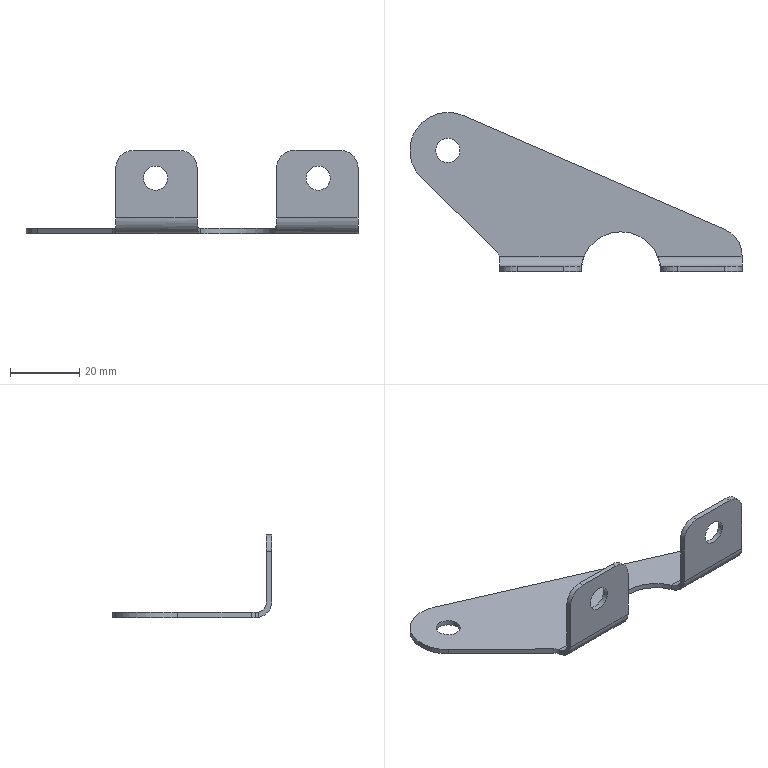Part | NX | features SKETCH 4, DATUM_CSYS 3, DATUM_PLANE 2, EXTRUDE 2, Flange 2, BLEND 1, Base Tab 1 | 1 solid | 35 faces | box 96 x 46 x 24 mm | volume 4607 mm3 | plane 16 | cylinder 15 | spline 4 | commonest cylinder face diameters 10 x4 6 x3 7 x3 9 x2 16 x1 22 x1
STEP:
#1=CARTESIAN_POINT('',(10.583,4.5,0.));
#2=VERTEX_POINT('',#1);
#3=CARTESIAN_POINT('',(-10.583,4.5,0.));
#4=VERTEX_POINT('',#3);
#5=CARTESIAN_POINT('',(0.,0.,0.));
#6=DIRECTION('',(0.,0.,1.));
#7=DIRECTION('',(1.,0.,0.));
#8=AXIS2_PLACEMENT_3D('',#5,#6,#7);
#9=CIRCLE('',#8,11.5);
#10=EDGE_CURVE('',#2,#4,#9,.T.);
#11=ORIENTED_EDGE('',*,*,#10,.F.);
#12=CARTESIAN_POINT('',(10.583,4.5,1.5));
#13=VERTEX_POINT('',#12);
#14=CARTESIAN_POINT('',(10.583,4.5,1.5));
#15=DIRECTION('',(0.,0.,-1.));
#16=VECTOR('',#15,1000.);
#17=LINE('',#14,#16);
#18=EDGE_CURVE('',#13,#2,#17,.T.);
#19=ORIENTED_EDGE('',*,*,#18,.F.);
#20=CARTESIAN_POINT('',(-10.583,4.5,1.5));
#21=VERTEX_POINT('',#20);
#22=CARTESIAN_POINT('',(0.,0.,1.5));
#23=DIRECTION('',(0.,0.,1.));
#24=DIRECTION('',(1.,0.,0.));
#25=AXIS2_PLACEMENT_3D('',#22,#23,#24);
#26=CIRCLE('',#25,11.5);
#27=EDGE_CURVE('',#13,#21,#26,.T.);
#28=ORIENTED_EDGE('',*,*,#27,.T.);
#29=CARTESIAN_POINT('',(-10.583,4.5,1.5));
#30=DIRECTION('',(0.,0.,-1.));
#31=VECTOR('',#30,1000.);
#32=LINE('',#29,#31);
#33=EDGE_CURVE('',#21,#4,#32,.T.);
#34=ORIENTED_EDGE('',*,*,#33,.T.);
#35=EDGE_LOOP('',(#11,#19,#28,#34));
#36=FACE_BOUND('',#35,.T.);
#37=CARTESIAN_POINT('',(0.,0.,1.5));
#38=DIRECTION('',(0.,0.,-1.));
#39=DIRECTION('',(-1.,0.,0.));
#40=AXIS2_PLACEMENT_3D('',#37,#38,#39);
#41=CYLINDRICAL_SURFACE('',#40,11.5);
#42=ADVANCED_FACE('',(#36),#41,.F.);
#43=CARTESIAN_POINT('',(35.,1.5,19.));
#44=VERTEX_POINT('',#43);
#45=CARTESIAN_POINT('',(35.,1.5,4.5));
#46=VERTEX_POINT('',#45);
#47=CARTESIAN_POINT('',(35.,1.5,24.));
#48=DIRECTION('',(0.,0.,-1.));
#49=VECTOR('',#48,1000.);
#50=LINE('',#47,#49);
#51=EDGE_CURVE('',#44,#46,#50,.T.);
#52=ORIENTED_EDGE('',*,*,#51,.F.);
#53=CARTESIAN_POINT('',(35.,0.,19.));
#54=VERTEX_POINT('',#53);
#55=CARTESIAN_POINT('',(35.,4.757,19.));
#56=DIRECTION('',(0.,1.,0.));
#57=VECTOR('',#56,1000.);
#58=LINE('',#55,#57);
#59=EDGE_CURVE('',#44,#54,#58,.F.);
#60=ORIENTED_EDGE('',*,*,#59,.T.);
#61=CARTESIAN_POINT('',(35.,0.,4.5));
#62=VERTEX_POINT('',#61);
#63=CARTESIAN_POINT('',(35.,0.,24.));
#64=DIRECTION('',(0.,0.,-1.));
#65=VECTOR('',#64,1000.);
#66=LINE('',#63,#65);
#67=EDGE_CURVE('',#54,#62,#66,.T.);
#68=ORIENTED_EDGE('',*,*,#67,.T.);
#69=CARTESIAN_POINT('',(35.,4.5,0.));
#70=VERTEX_POINT('',#69);
#71=CARTESIAN_POINT('',(35.,4.5,4.5));
#72=DIRECTION('',(-1.,0.,0.));
#73=DIRECTION('',(0.,0.,1.));
#74=AXIS2_PLACEMENT_3D('',#71,#72,#73);
#75=CIRCLE('',#74,4.5);
#76=EDGE_CURVE('',#70,#62,#75,.T.);
#77=ORIENTED_EDGE('',*,*,#76,.F.);
#78=CARTESIAN_POINT('',(35.,4.757,0.));
#79=VERTEX_POINT('',#78);
#80=CARTESIAN_POINT('',(35.,4.757,0.));
#81=DIRECTION('',(0.,-1.,0.));
#82=VECTOR('',#81,1000.);
#83=LINE('',#80,#82);
#84=EDGE_CURVE('',#79,#70,#83,.T.);
#85=ORIENTED_EDGE('',*,*,#84,.F.);
#86=CARTESIAN_POINT('',(35.,4.757,1.5));
#87=VERTEX_POINT('',#86);
#88=CARTESIAN_POINT('',(35.,4.757,1.5));
#89=DIRECTION('',(0.,0.,-1.));
#90=VECTOR('',#89,1000.);
#91=LINE('',#88,#90);
#92=EDGE_CURVE('',#87,#79,#91,.T.);
#93=ORIENTED_EDGE('',*,*,#92,.F.);
#94=CARTESIAN_POINT('',(35.,4.5,1.5));
#95=VERTEX_POINT('',#94);
#96=CARTESIAN_POINT('',(35.,4.757,1.5));
#97=DIRECTION('',(0.,-1.,0.));
#98=VECTOR('',#97,1000.);
#99=LINE('',#96,#98);
#100=EDGE_CURVE('',#87,#95,#99,.T.);
#101=ORIENTED_EDGE('',*,*,#100,.T.);
#102=CARTESIAN_POINT('',(35.,4.5,4.5));
#103=DIRECTION('',(-1.,0.,0.));
#104=DIRECTION('',(0.,-1.,0.));
#105=AXIS2_PLACEMENT_3D('',#102,#103,#104);
#106=CIRCLE('',#105,3.);
#107=EDGE_CURVE('',#95,#46,#106,.T.);
#108=ORIENTED_EDGE('',*,*,#107,.T.);
#109=EDGE_LOOP('',(#52,#60,#68,#77,#85,#93,#101,#108));
#110=FACE_BOUND('',#109,.T.);
#111=CARTESIAN_POINT('',(35.,4.757,1.5));
#112=DIRECTION('',(1.,0.,0.));
#113=DIRECTION('',(0.,0.,-1.));
#114=AXIS2_PLACEMENT_3D('',#111,#112,#113);
#115=PLANE('',#114);
#116=ADVANCED_FACE('',(#110),#115,.T.);
#117=CARTESIAN_POINT('',(-46.5,35.,0.));
#118=VERTEX_POINT('',#117);
#119=CARTESIAN_POINT('',(-50.,35.,0.));
#120=DIRECTION('',(0.,0.,1.));
#121=DIRECTION('',(1.,0.,0.));
#122=AXIS2_PLACEMENT_3D('',#119,#120,#121);
#123=CIRCLE('',#122,3.5);
#124=EDGE_CURVE('',#118,#118,#123,.T.);
#125=ORIENTED_EDGE('',*,*,#124,.T.);
#126=EDGE_LOOP('',(#125));
#127=FACE_BOUND('',#126,.T.);
#128=ORIENTED_EDGE('',*,*,#84,.T.);
#129=CARTESIAN_POINT('',(35.,4.5,0.));
#130=DIRECTION('',(-1.,0.,0.));
#131=VECTOR('',#130,1000.);
#132=LINE('',#129,#131);
#133=EDGE_CURVE('',#70,#2,#132,.T.);
#134=ORIENTED_EDGE('',*,*,#133,.T.);
#135=ORIENTED_EDGE('',*,*,#10,.T.);
#136=CARTESIAN_POINT('',(-35.,4.5,0.));
#137=VERTEX_POINT('',#136);
#138=CARTESIAN_POINT('',(-35.002,4.5,0.));
#139=DIRECTION('',(-1.,0.,0.));
#140=VECTOR('',#139,1000.);
#141=LINE('',#138,#140);
#142=EDGE_CURVE('',#4,#137,#141,.T.);
#143=ORIENTED_EDGE('',*,*,#142,.T.);
#144=CARTESIAN_POINT('',(-35.002,4.5,0.));
#145=VERTEX_POINT('',#144);
#146=CARTESIAN_POINT('',(-35.002,4.5,0.));
#147=DIRECTION('',(-1.,0.,0.));
#148=VECTOR('',#147,1000.);
#149=LINE('',#146,#148);
#150=EDGE_CURVE('',#137,#145,#149,.T.);
#151=ORIENTED_EDGE('',*,*,#150,.T.);
#152=CARTESIAN_POINT('',(-35.002,3.845,0.));
#153=VERTEX_POINT('',#152);
#154=CARTESIAN_POINT('',(-35.002,0.,0.));
#155=DIRECTION('',(0.,-1.,0.));
#156=VECTOR('',#155,1000.);
#157=LINE('',#154,#156);
#158=EDGE_CURVE('',#145,#153,#157,.T.);
#159=ORIENTED_EDGE('',*,*,#158,.T.);
#160=CARTESIAN_POINT('',(-35.905,5.883,0.));
#161=VERTEX_POINT('',#160);
#162=CARTESIAN_POINT('',(-38.,3.736,0.));
#163=DIRECTION('',(0.,0.,1.));
#164=DIRECTION('',(1.,0.,0.));
#165=AXIS2_PLACEMENT_3D('',#162,#163,#164);
#166=CIRCLE('',#165,3.);
#167=EDGE_CURVE('',#153,#161,#166,.T.);
#168=ORIENTED_EDGE('',*,*,#167,.T.);
#169=CARTESIAN_POINT('',(-57.681,27.126,0.));
#170=VERTEX_POINT('',#169);
#171=CARTESIAN_POINT('',(-35.905,5.883,0.));
#172=DIRECTION('',(-0.7158,0.6983,0.));
#173=VECTOR('',#172,1000.);
#174=LINE('',#171,#173);
#175=EDGE_CURVE('',#161,#170,#174,.T.);
#176=ORIENTED_EDGE('',*,*,#175,.T.);
#177=CARTESIAN_POINT('',(-45.61,45.086,0.));
#178=VERTEX_POINT('',#177);
#179=CARTESIAN_POINT('',(-50.,35.,0.));
#180=DIRECTION('',(0.,0.,-1.));
#181=DIRECTION('',(1.,0.,0.));
#182=AXIS2_PLACEMENT_3D('',#179,#180,#181);
#183=CIRCLE('',#182,11.);
#184=EDGE_CURVE('',#170,#178,#183,.T.);
#185=ORIENTED_EDGE('',*,*,#184,.T.);
#186=CARTESIAN_POINT('',(30.193,12.092,0.));
#187=VERTEX_POINT('',#186);
#188=CARTESIAN_POINT('',(-45.61,45.086,0.));
#189=DIRECTION('',(0.9169,-0.3991,0.));
#190=VECTOR('',#189,1000.);
#191=LINE('',#188,#190);
#192=EDGE_CURVE('',#178,#187,#191,.T.);
#193=ORIENTED_EDGE('',*,*,#192,.T.);
#194=CARTESIAN_POINT('',(27.,4.757,0.));
#195=DIRECTION('',(0.,0.,-1.));
#196=DIRECTION('',(1.,0.,0.));
#197=AXIS2_PLACEMENT_3D('',#194,#195,#196);
#198=CIRCLE('',#197,8.);
#199=EDGE_CURVE('',#187,#79,#198,.T.);
#200=ORIENTED_EDGE('',*,*,#199,.T.);
#201=EDGE_LOOP('',(#128,#134,#135,#143,#151,#159,#168,#176,#185,#193,#200));
#202=FACE_BOUND('',#201,.T.);
#203=CARTESIAN_POINT('',(-50.,35.,0.));
#204=DIRECTION('',(0.,0.,-1.));
#205=DIRECTION('',(-1.,0.,0.));
#206=AXIS2_PLACEMENT_3D('',#203,#204,#205);
#207=PLANE('',#206);
#208=ADVANCED_FACE('',(#127,#202),#207,.T.);
#209=ORIENTED_EDGE('',*,*,#175,.F.);
#210=CARTESIAN_POINT('',(-35.905,5.883,1.5));
#211=VERTEX_POINT('',#210);
#212=CARTESIAN_POINT('',(-35.905,5.883,1.5));
#213=DIRECTION('',(0.,0.,-1.));
#214=VECTOR('',#213,1000.);
#215=LINE('',#212,#214);
#216=EDGE_CURVE('',#211,#161,#215,.T.);
#217=ORIENTED_EDGE('',*,*,#216,.F.);
#218=CARTESIAN_POINT('',(-57.681,27.126,1.5));
#219=VERTEX_POINT('',#218);
#220=CARTESIAN_POINT('',(-35.905,5.883,1.5));
#221=DIRECTION('',(-0.7158,0.6983,0.));
#222=VECTOR('',#221,1000.);
#223=LINE('',#220,#222);
#224=EDGE_CURVE('',#211,#219,#223,.T.);
#225=ORIENTED_EDGE('',*,*,#224,.T.);
#226=CARTESIAN_POINT('',(-57.681,27.126,1.5));
#227=DIRECTION('',(0.,0.,-1.));
#228=VECTOR('',#227,1000.);
#229=LINE('',#226,#228);
#230=EDGE_CURVE('',#219,#170,#229,.T.);
#231=ORIENTED_EDGE('',*,*,#230,.T.);
#232=EDGE_LOOP('',(#209,#217,#225,#231));
#233=FACE_BOUND('',#232,.T.);
#234=CARTESIAN_POINT('',(-35.905,5.883,1.5));
#235=DIRECTION('',(-0.6983,-0.7158,0.));
#236=DIRECTION('',(0.7158,-0.6983,0.));
#237=AXIS2_PLACEMENT_3D('',#234,#235,#236);
#238=PLANE('',#237);
#239=ADVANCED_FACE('',(#233),#238,.T.);
#240=ORIENTED_EDGE('',*,*,#184,.F.);
#241=ORIENTED_EDGE('',*,*,#230,.F.);
#242=CARTESIAN_POINT('',(-45.61,45.086,1.5));
#243=VERTEX_POINT('',#242);
#244=CARTESIAN_POINT('',(-50.,35.,1.5));
#245=DIRECTION('',(0.,0.,-1.));
#246=DIRECTION('',(1.,0.,0.));
#247=AXIS2_PLACEMENT_3D('',#244,#245,#246);
#248=CIRCLE('',#247,11.);
#249=EDGE_CURVE('',#219,#243,#248,.T.);
#250=ORIENTED_EDGE('',*,*,#249,.T.);
#251=CARTESIAN_POINT('',(-45.61,45.086,1.5));
#252=DIRECTION('',(0.,0.,-1.));
#253=VECTOR('',#252,1000.);
#254=LINE('',#251,#253);
#255=EDGE_CURVE('',#243,#178,#254,.T.);
#256=ORIENTED_EDGE('',*,*,#255,.T.);
#257=EDGE_LOOP('',(#240,#241,#250,#256));
#258=FACE_BOUND('',#257,.T.);
#259=CARTESIAN_POINT('',(-50.,35.,1.5));
#260=DIRECTION('',(0.,0.,-1.));
#261=DIRECTION('',(-1.,0.,0.));
#262=AXIS2_PLACEMENT_3D('',#259,#260,#261);
#263=CYLINDRICAL_SURFACE('',#262,11.);
#264=ADVANCED_FACE('',(#258),#263,.T.);
#265=ORIENTED_EDGE('',*,*,#192,.F.);
#266=ORIENTED_EDGE('',*,*,#255,.F.);
#267=CARTESIAN_POINT('',(30.193,12.092,1.5));
#268=VERTEX_POINT('',#267);
#269=CARTESIAN_POINT('',(-45.61,45.086,1.5));
#270=DIRECTION('',(0.9169,-0.3991,0.));
#271=VECTOR('',#270,1000.);
#272=LINE('',#269,#271);
#273=EDGE_CURVE('',#243,#268,#272,.T.);
#274=ORIENTED_EDGE('',*,*,#273,.T.);
#275=CARTESIAN_POINT('',(30.193,12.092,1.5));
#276=DIRECTION('',(0.,0.,-1.));
#277=VECTOR('',#276,1000.);
#278=LINE('',#275,#277);
#279=EDGE_CURVE('',#268,#187,#278,.T.);
#280=ORIENTED_EDGE('',*,*,#279,.T.);
#281=EDGE_LOOP('',(#265,#266,#274,#280));
#282=FACE_BOUND('',#281,.T.);
#283=CARTESIAN_POINT('',(-45.61,45.086,1.5));
#284=DIRECTION('',(0.3991,0.9169,0.));
#285=DIRECTION('',(-0.9169,0.3991,0.));
#286=AXIS2_PLACEMENT_3D('',#283,#284,#285);
#287=PLANE('',#286);
#288=ADVANCED_FACE('',(#282),#287,.T.);
#289=ORIENTED_EDGE('',*,*,#199,.F.);
#290=ORIENTED_EDGE('',*,*,#279,.F.);
#291=CARTESIAN_POINT('',(27.,4.757,1.5));
#292=DIRECTION('',(0.,0.,-1.));
#293=DIRECTION('',(1.,0.,0.));
#294=AXIS2_PLACEMENT_3D('',#291,#292,#293);
#295=CIRCLE('',#294,8.);
#296=EDGE_CURVE('',#268,#87,#295,.T.);
#297=ORIENTED_EDGE('',*,*,#296,.T.);
#298=ORIENTED_EDGE('',*,*,#92,.T.);
#299=EDGE_LOOP('',(#289,#290,#297,#298));
#300=FACE_BOUND('',#299,.T.);
#301=CARTESIAN_POINT('',(27.,4.757,1.5));
#302=DIRECTION('',(0.,0.,-1.));
#303=DIRECTION('',(-1.,0.,0.));
#304=AXIS2_PLACEMENT_3D('',#301,#302,#303);
#305=CYLINDRICAL_SURFACE('',#304,8.);
#306=ADVANCED_FACE('',(#300),#305,.T.);
#307=CARTESIAN_POINT('',(-35.002,3.845,1.5));
#308=VERTEX_POINT('',#307);
#309=CARTESIAN_POINT('',(-35.002,3.845,1.5));
#310=DIRECTION('',(0.,0.,-1.));
#311=VECTOR('',#310,1000.);
#312=LINE('',#309,#311);
#313=EDGE_CURVE('',#308,#153,#312,.T.);
#314=ORIENTED_EDGE('',*,*,#313,.F.);
#315=CARTESIAN_POINT('',(-38.,3.736,1.5));
#316=DIRECTION('',(0.,0.,1.));
#317=DIRECTION('',(1.,0.,0.));
#318=AXIS2_PLACEMENT_3D('',#315,#316,#317);
#319=CIRCLE('',#318,3.);
#320=EDGE_CURVE('',#308,#211,#319,.T.);
#321=ORIENTED_EDGE('',*,*,#320,.T.);
#322=ORIENTED_EDGE('',*,*,#216,.T.);
#323=ORIENTED_EDGE('',*,*,#167,.F.);
#324=EDGE_LOOP('',(#314,#321,#322,#323));
#325=FACE_BOUND('',#324,.T.);
#326=CARTESIAN_POINT('',(-38.,3.736,1.5));
#327=DIRECTION('',(0.,0.,-1.));
#328=DIRECTION('',(-1.,0.,0.));
#329=AXIS2_PLACEMENT_3D('',#326,#327,#328);
#330=CYLINDRICAL_SURFACE('',#329,3.);
#331=ADVANCED_FACE('',(#325),#330,.F.);
#332=CARTESIAN_POINT('',(-53.5,35.,1.5));
#333=VERTEX_POINT('',#332);
#334=CARTESIAN_POINT('',(-50.,35.,1.5));
#335=DIRECTION('',(0.,0.,-1.));
#336=DIRECTION('',(-1.,0.,0.));
#337=AXIS2_PLACEMENT_3D('',#334,#335,#336);
#338=CIRCLE('',#337,3.5);
#339=EDGE_CURVE('',#333,#333,#338,.F.);
#340=ORIENTED_EDGE('',*,*,#339,.F.);
#341=EDGE_LOOP('',(#340));
#342=FACE_BOUND('',#341,.T.);
#343=CARTESIAN_POINT('',(35.,4.5,1.5));
#344=DIRECTION('',(-1.,0.,0.));
#345=VECTOR('',#344,1000.);
#346=LINE('',#343,#345);
#347=EDGE_CURVE('',#95,#13,#346,.T.);
#348=ORIENTED_EDGE('',*,*,#347,.F.);
#349=ORIENTED_EDGE('',*,*,#100,.F.);
#350=ORIENTED_EDGE('',*,*,#296,.F.);
#351=ORIENTED_EDGE('',*,*,#273,.F.);
#352=ORIENTED_EDGE('',*,*,#249,.F.);
#353=ORIENTED_EDGE('',*,*,#224,.F.);
#354=ORIENTED_EDGE('',*,*,#320,.F.);
#355=CARTESIAN_POINT('',(-35.002,4.5,1.5));
#356=VERTEX_POINT('',#355);
#357=CARTESIAN_POINT('',(-35.002,4.5,1.5));
#358=DIRECTION('',(0.,1.,0.));
#359=VECTOR('',#358,1000.);
#360=LINE('',#357,#359);
#361=EDGE_CURVE('',#356,#308,#360,.F.);
#362=ORIENTED_EDGE('',*,*,#361,.F.);
#363=CARTESIAN_POINT('',(-35.,4.5,1.5));
#364=VERTEX_POINT('',#363);
#365=CARTESIAN_POINT('',(-35.,4.5,1.5));
#366=DIRECTION('',(1.,0.,0.));
#367=VECTOR('',#366,1000.);
#368=LINE('',#365,#367);
#369=EDGE_CURVE('',#364,#356,#368,.F.);
#370=ORIENTED_EDGE('',*,*,#369,.F.);
#371=CARTESIAN_POINT('',(-35.,4.5,1.5));
#372=DIRECTION('',(1.,0.,0.));
#373=VECTOR('',#372,1000.);
#374=LINE('',#371,#373);
#375=EDGE_CURVE('',#21,#364,#374,.F.);
#376=ORIENTED_EDGE('',*,*,#375,.F.);
#377=ORIENTED_EDGE('',*,*,#27,.F.);
#378=EDGE_LOOP('',(#348,#349,#350,#351,#352,#353,#354,#362,#370,#376,#377));
#379=FACE_BOUND('',#378,.T.);
#380=CARTESIAN_POINT('',(-50.,35.,1.5));
#381=DIRECTION('',(0.,0.,-1.));
#382=DIRECTION('',(-1.,0.,0.));
#383=AXIS2_PLACEMENT_3D('',#380,#381,#382);
#384=PLANE('',#383);
#385=ADVANCED_FACE('',(#342,#379),#384,.F.);
#386=ORIENTED_EDGE('',*,*,#313,.T.);
#387=ORIENTED_EDGE('',*,*,#158,.F.);
#388=CARTESIAN_POINT('',(-35.002,4.5,0.));
#389=DIRECTION('',(0.,0.,-1.));
#390=VECTOR('',#389,1000.);
#391=LINE('',#388,#390);
#392=EDGE_CURVE('',#356,#145,#391,.T.);
#393=ORIENTED_EDGE('',*,*,#392,.F.);
#394=ORIENTED_EDGE('',*,*,#361,.T.);
#395=EDGE_LOOP('',(#386,#387,#393,#394));
#396=FACE_BOUND('',#395,.T.);
#397=CARTESIAN_POINT('',(-35.002,0.,0.));
#398=DIRECTION('',(-1.,0.,0.));
#399=DIRECTION('',(0.,-1.,0.));
#400=AXIS2_PLACEMENT_3D('',#397,#398,#399);
#401=PLANE('',#400);
#402=ADVANCED_FACE('',(#396),#401,.F.);
#403=ORIENTED_EDGE('',*,*,#150,.F.);
#404=CARTESIAN_POINT('',(-35.,4.5,0.));
#405=DIRECTION('',(0.,0.,-1.));
#406=VECTOR('',#405,1000.);
#407=LINE('',#404,#406);
#408=EDGE_CURVE('',#364,#137,#407,.T.);
#409=ORIENTED_EDGE('',*,*,#408,.F.);
#410=ORIENTED_EDGE('',*,*,#369,.T.);
#411=ORIENTED_EDGE('',*,*,#392,.T.);
#412=EDGE_LOOP('',(#403,#409,#410,#411));
#413=FACE_BOUND('',#412,.T.);
#414=CARTESIAN_POINT('',(-35.002,4.5,0.));
#415=DIRECTION('',(0.,1.,0.));
#416=DIRECTION('',(-1.,0.,0.));
#417=AXIS2_PLACEMENT_3D('',#414,#415,#416);
#418=PLANE('',#417);
#419=ADVANCED_FACE('',(#413),#418,.F.);
#420=CARTESIAN_POINT('',(-11.5,1.5,19.));
#421=VERTEX_POINT('',#420);
#422=CARTESIAN_POINT('',(-11.5,1.5,4.5));
#423=VERTEX_POINT('',#422);
#424=CARTESIAN_POINT('',(-11.5,1.5,24.));
#425=DIRECTION('',(0.,0.,-1.));
#426=VECTOR('',#425,1000.);
#427=LINE('',#424,#426);
#428=EDGE_CURVE('',#421,#423,#427,.T.);
#429=ORIENTED_EDGE('',*,*,#428,.F.);
#430=CARTESIAN_POINT('',(-11.5,0.,19.));
#431=VERTEX_POINT('',#430);
#432=CARTESIAN_POINT('',(-11.5,0.,19.));
#433=DIRECTION('',(0.,1.,0.));
#434=VECTOR('',#433,1000.);
#435=LINE('',#432,#434);
#436=EDGE_CURVE('',#421,#431,#435,.F.);
#437=ORIENTED_EDGE('',*,*,#436,.T.);
#438=CARTESIAN_POINT('',(-11.5,0.,4.5));
#439=VERTEX_POINT('',#438);
#440=CARTESIAN_POINT('',(-11.5,0.,24.));
#441=DIRECTION('',(0.,0.,-1.));
#442=VECTOR('',#441,1000.);
#443=LINE('',#440,#442);
#444=EDGE_CURVE('',#431,#439,#443,.T.);
#445=ORIENTED_EDGE('',*,*,#444,.T.);
#446=CARTESIAN_POINT('',(-11.5,1.5,4.5));
#447=DIRECTION('',(0.,-1.,0.));
#448=VECTOR('',#447,1000.);
#449=LINE('',#446,#448);
#450=EDGE_CURVE('',#423,#439,#449,.T.);
#451=ORIENTED_EDGE('',*,*,#450,.F.);
#452=EDGE_LOOP('',(#429,#437,#445,#451));
#453=FACE_BOUND('',#452,.T.);
#454=CARTESIAN_POINT('',(-11.5,0.,24.));
#455=DIRECTION('',(1.,0.,0.));
#456=DIRECTION('',(0.,1.,0.));
#457=AXIS2_PLACEMENT_3D('',#454,#455,#456);
#458=PLANE('',#457);
#459=ADVANCED_FACE('',(#453),#458,.T.);
#460=CARTESIAN_POINT('',(-35.,0.,4.5));
#461=VERTEX_POINT('',#460);
#462=CARTESIAN_POINT('',(-35.,0.,19.));
#463=VERTEX_POINT('',#462);
#464=CARTESIAN_POINT('',(-35.,0.,1.755));
#465=DIRECTION('',(0.,0.,1.));
#466=VECTOR('',#465,1000.);
#467=LINE('',#464,#466);
#468=EDGE_CURVE('',#461,#463,#467,.T.);
#469=ORIENTED_EDGE('',*,*,#468,.T.);
#470=CARTESIAN_POINT('',(-35.,1.5,19.));
#471=VERTEX_POINT('',#470);
#472=CARTESIAN_POINT('',(-35.,0.,19.));
#473=DIRECTION('',(0.,1.,0.));
#474=VECTOR('',#473,1000.);
#475=LINE('',#472,#474);
#476=EDGE_CURVE('',#463,#471,#475,.T.);
#477=ORIENTED_EDGE('',*,*,#476,.T.);
#478=CARTESIAN_POINT('',(-35.,1.5,4.5));
#479=VERTEX_POINT('',#478);
#480=CARTESIAN_POINT('',(-35.,1.5,1.755));
#481=DIRECTION('',(0.,0.,1.));
#482=VECTOR('',#481,1000.);
#483=LINE('',#480,#482);
#484=EDGE_CURVE('',#479,#471,#483,.T.);
#485=ORIENTED_EDGE('',*,*,#484,.F.);
#486=CARTESIAN_POINT('',(-35.,4.5,4.5));
#487=DIRECTION('',(-1.,0.,0.));
#488=DIRECTION('',(0.,-1.,0.));
#489=AXIS2_PLACEMENT_3D('',#486,#487,#488);
#490=CIRCLE('',#489,3.);
#491=EDGE_CURVE('',#479,#364,#490,.F.);
#492=ORIENTED_EDGE('',*,*,#491,.T.);
#493=ORIENTED_EDGE('',*,*,#408,.T.);
#494=CARTESIAN_POINT('',(-35.,4.5,4.5));
#495=DIRECTION('',(1.,0.,0.));
#496=DIRECTION('',(0.,0.,1.));
#497=AXIS2_PLACEMENT_3D('',#494,#495,#496);
#498=CIRCLE('',#497,4.5);
#499=EDGE_CURVE('',#461,#137,#498,.T.);
#500=ORIENTED_EDGE('',*,*,#499,.F.);
#501=EDGE_LOOP('',(#469,#477,#485,#492,#493,#500));
#502=FACE_BOUND('',#501,.T.);
#503=CARTESIAN_POINT('',(-35.,0.,1.755));
#504=DIRECTION('',(-1.,0.,0.));
#505=DIRECTION('',(0.,-1.,0.));
#506=AXIS2_PLACEMENT_3D('',#503,#504,#505);
#507=PLANE('',#506);
#508=ADVANCED_FACE('',(#502),#507,.T.);
#509=CARTESIAN_POINT('',(-20.,0.,16.));
#510=VERTEX_POINT('',#509);
#511=CARTESIAN_POINT('',(-23.5,0.,16.));
#512=DIRECTION('',(0.,-1.,0.));
#513=DIRECTION('',(1.,0.,0.));
#514=AXIS2_PLACEMENT_3D('',#511,#512,#513);
#515=CIRCLE('',#514,3.5);
#516=EDGE_CURVE('',#510,#510,#515,.T.);
#517=ORIENTED_EDGE('',*,*,#516,.F.);
#518=EDGE_LOOP('',(#517));
#519=FACE_BOUND('',#518,.T.);
#520=ORIENTED_EDGE('',*,*,#444,.F.);
#521=CARTESIAN_POINT('',(-16.5,0.,24.));
#522=VERTEX_POINT('',#521);
#523=CARTESIAN_POINT('',(-16.5,0.,19.));
#524=DIRECTION('',(0.,1.,0.));
#525=DIRECTION('',(-1.,0.,0.));
#526=AXIS2_PLACEMENT_3D('',#523,#524,#525);
#527=CIRCLE('',#526,5.);
#528=EDGE_CURVE('',#431,#522,#527,.F.);
#529=ORIENTED_EDGE('',*,*,#528,.T.);
#530=CARTESIAN_POINT('',(-30.,0.,24.));
#531=VERTEX_POINT('',#530);
#532=CARTESIAN_POINT('',(-35.,0.,24.));
#533=DIRECTION('',(1.,0.,0.));
#534=VECTOR('',#533,1000.);
#535=LINE('',#532,#534);
#536=EDGE_CURVE('',#531,#522,#535,.T.);
#537=ORIENTED_EDGE('',*,*,#536,.F.);
#538=CARTESIAN_POINT('',(-30.,0.,19.));
#539=DIRECTION('',(0.,1.,0.));
#540=DIRECTION('',(-1.,0.,0.));
#541=AXIS2_PLACEMENT_3D('',#538,#539,#540);
#542=CIRCLE('',#541,5.);
#543=EDGE_CURVE('',#531,#463,#542,.F.);
#544=ORIENTED_EDGE('',*,*,#543,.T.);
#545=ORIENTED_EDGE('',*,*,#468,.F.);
#546=CARTESIAN_POINT('',(-35.,0.,4.5));
#547=DIRECTION('',(1.,0.,0.));
#548=VECTOR('',#547,1000.);
#549=LINE('',#546,#548);
#550=EDGE_CURVE('',#461,#439,#549,.T.);
#551=ORIENTED_EDGE('',*,*,#550,.T.);
#552=EDGE_LOOP('',(#520,#529,#537,#544,#545,#551));
#553=FACE_BOUND('',#552,.T.);
#554=CARTESIAN_POINT('',(0.,0.,0.));
#555=DIRECTION('',(0.,1.,0.));
#556=DIRECTION('',(-1.,0.,0.));
#557=AXIS2_PLACEMENT_3D('',#554,#555,#556);
#558=PLANE('',#557);
#559=ADVANCED_FACE('',(#519,#553),#558,.F.);
#560=CARTESIAN_POINT('',(-27.,1.5,16.));
#561=VERTEX_POINT('',#560);
#562=CARTESIAN_POINT('',(-23.5,1.5,16.));
#563=DIRECTION('',(0.,1.,0.));
#564=DIRECTION('',(-1.,0.,0.));
#565=AXIS2_PLACEMENT_3D('',#562,#563,#564);
#566=CIRCLE('',#565,3.5);
#567=EDGE_CURVE('',#561,#561,#566,.T.);
#568=ORIENTED_EDGE('',*,*,#567,.F.);
#569=EDGE_LOOP('',(#568));
#570=FACE_BOUND('',#569,.T.);
#571=CARTESIAN_POINT('',(-30.,1.5,24.));
#572=VERTEX_POINT('',#571);
#573=CARTESIAN_POINT('',(-16.5,1.5,24.));
#574=VERTEX_POINT('',#573);
#575=CARTESIAN_POINT('',(-35.,1.5,24.));
#576=DIRECTION('',(1.,0.,0.));
#577=VECTOR('',#576,1000.);
#578=LINE('',#575,#577);
#579=EDGE_CURVE('',#572,#574,#578,.T.);
#580=ORIENTED_EDGE('',*,*,#579,.T.);
#581=CARTESIAN_POINT('',(-16.5,1.5,19.));
#582=DIRECTION('',(0.,1.,0.));
#583=DIRECTION('',(-1.,0.,0.));
#584=AXIS2_PLACEMENT_3D('',#581,#582,#583);
#585=CIRCLE('',#584,5.);
#586=EDGE_CURVE('',#574,#421,#585,.T.);
#587=ORIENTED_EDGE('',*,*,#586,.T.);
#588=ORIENTED_EDGE('',*,*,#428,.T.);
#589=CARTESIAN_POINT('',(-35.,1.5,4.5));
#590=DIRECTION('',(1.,0.,0.));
#591=VECTOR('',#590,1000.);
#592=LINE('',#589,#591);
#593=EDGE_CURVE('',#479,#423,#592,.T.);
#594=ORIENTED_EDGE('',*,*,#593,.F.);
#595=ORIENTED_EDGE('',*,*,#484,.T.);
#596=CARTESIAN_POINT('',(-30.,1.5,19.));
#597=DIRECTION('',(0.,1.,0.));
#598=DIRECTION('',(-1.,0.,0.));
#599=AXIS2_PLACEMENT_3D('',#596,#597,#598);
#600=CIRCLE('',#599,5.);
#601=EDGE_CURVE('',#471,#572,#600,.T.);
#602=ORIENTED_EDGE('',*,*,#601,.T.);
#603=EDGE_LOOP('',(#580,#587,#588,#594,#595,#602));
#604=FACE_BOUND('',#603,.T.);
#605=CARTESIAN_POINT('',(0.,1.5,0.));
#606=DIRECTION('',(0.,1.,0.));
#607=DIRECTION('',(-1.,0.,0.));
#608=AXIS2_PLACEMENT_3D('',#605,#606,#607);
#609=PLANE('',#608);
#610=ADVANCED_FACE('',(#570,#604),#609,.T.);
#611=ORIENTED_EDGE('',*,*,#536,.T.);
#612=CARTESIAN_POINT('',(-16.5,0.,24.));
#613=DIRECTION('',(0.,1.,0.));
#614=VECTOR('',#613,1000.);
#615=LINE('',#612,#614);
#616=EDGE_CURVE('',#522,#574,#615,.T.);
#617=ORIENTED_EDGE('',*,*,#616,.T.);
#618=ORIENTED_EDGE('',*,*,#579,.F.);
#619=CARTESIAN_POINT('',(-30.,0.,24.));
#620=DIRECTION('',(0.,1.,0.));
#621=VECTOR('',#620,1000.);
#622=LINE('',#619,#621);
#623=EDGE_CURVE('',#572,#531,#622,.F.);
#624=ORIENTED_EDGE('',*,*,#623,.T.);
#625=EDGE_LOOP('',(#611,#617,#618,#624));
#626=FACE_BOUND('',#625,.T.);
#627=CARTESIAN_POINT('',(-35.,0.,24.));
#628=DIRECTION('',(0.,0.,1.));
#629=DIRECTION('',(1.,0.,0.));
#630=AXIS2_PLACEMENT_3D('',#627,#628,#629);
#631=PLANE('',#630);
#632=ADVANCED_FACE('',(#626),#631,.T.);
#633=CARTESIAN_POINT('',(-11.365,2.379,2.379));
#634=VERTEX_POINT('',#633);
#635=CARTESIAN_POINT('',(-10.583,4.5,1.5));
#636=CARTESIAN_POINT('',(-10.956,3.747,1.5));
#637=CARTESIAN_POINT('',(-11.22,2.951,1.806));
#638=CARTESIAN_POINT('',(-11.365,2.379,2.379));
#639=B_SPLINE_CURVE_WITH_KNOTS('',3,(#635,#636,#637,#638),.UNSPECIFIED.,.F.,.F.,(4,4),(2.74,2.988),.UNSPECIFIED.);
#640=EDGE_CURVE('',#21,#634,#639,.T.);
#641=ORIENTED_EDGE('',*,*,#640,.T.);
#642=CARTESIAN_POINT('',(-11.365,1.318,1.318));
#643=VERTEX_POINT('',#642);
#644=CARTESIAN_POINT('',(-11.365,1.318,1.318));
#645=DIRECTION('',(0.,-0.7071,-0.7071));
#646=VECTOR('',#645,1000.);
#647=LINE('',#644,#646);
#648=EDGE_CURVE('',#634,#643,#647,.T.);
#649=ORIENTED_EDGE('',*,*,#648,.T.);
#650=CARTESIAN_POINT('',(-10.583,4.5,0.));
#651=CARTESIAN_POINT('',(-10.956,3.37,0.));
#652=CARTESIAN_POINT('',(-11.22,2.176,0.4597));
#653=CARTESIAN_POINT('',(-11.365,1.318,1.318));
#654=B_SPLINE_CURVE_WITH_KNOTS('',3,(#650,#651,#652,#653),.UNSPECIFIED.,.F.,.F.,(4,4),(2.74,2.988),.UNSPECIFIED.);
#655=EDGE_CURVE('',#4,#643,#654,.T.);
#656=ORIENTED_EDGE('',*,*,#655,.F.);
#657=ORIENTED_EDGE('',*,*,#33,.F.);
#658=EDGE_LOOP('',(#641,#649,#656,#657));
#659=FACE_BOUND('',#658,.T.);
#660=CARTESIAN_POINT('',(-10.583,4.5,0.));
#661=CARTESIAN_POINT('',(-10.77,3.935,0.));
#662=CARTESIAN_POINT('',(-10.929,3.354,0.1084));
#663=CARTESIAN_POINT('',(-11.19,2.26,0.5528));
#664=CARTESIAN_POINT('',(-11.292,1.747,0.8886));
#665=CARTESIAN_POINT('',(-11.365,1.318,1.318));
#666=CARTESIAN_POINT('',(-10.583,4.5,1.5));
#667=CARTESIAN_POINT('',(-10.77,4.123,1.5));
#668=CARTESIAN_POINT('',(-10.929,3.736,1.572));
#669=CARTESIAN_POINT('',(-11.19,3.007,1.869));
#670=CARTESIAN_POINT('',(-11.292,2.665,2.092));
#671=CARTESIAN_POINT('',(-11.365,2.379,2.379));
#672=B_SPLINE_SURFACE_WITH_KNOTS('',1,3,((#660,#661,#662,#663,#664,#665),(#666,#667,#668,#669,#670,#671)),.RULED_SURF.,.F.,.F.,.F.,(2,2),(4,2,4),(0.,1.),(2.74,2.864,2.988),.UNSPECIFIED.);
#673=ADVANCED_FACE('',(#659),#672,.T.);
#674=ORIENTED_EDGE('',*,*,#142,.F.);
#675=ORIENTED_EDGE('',*,*,#655,.T.);
#676=CARTESIAN_POINT('',(-11.365,1.318,1.318));
#677=CARTESIAN_POINT('',(-11.41,0.485,2.151));
#678=CARTESIAN_POINT('',(-11.455,0.,3.322));
#679=CARTESIAN_POINT('',(-11.5,0.,4.5));
#680=B_SPLINE_CURVE_WITH_KNOTS('',3,(#676,#677,#678,#679),.UNSPECIFIED.,.F.,.F.,(4,4),(0.,1.),.UNSPECIFIED.);
#681=EDGE_CURVE('',#643,#439,#680,.T.);
#682=ORIENTED_EDGE('',*,*,#681,.T.);
#683=ORIENTED_EDGE('',*,*,#550,.F.);
#684=ORIENTED_EDGE('',*,*,#499,.T.);
#685=EDGE_LOOP('',(#674,#675,#682,#683,#684));
#686=FACE_BOUND('',#685,.T.);
#687=CARTESIAN_POINT('',(-10.583,4.5,4.5));
#688=DIRECTION('',(-1.,0.,0.));
#689=DIRECTION('',(0.,0.,1.));
#690=AXIS2_PLACEMENT_3D('',#687,#688,#689);
#691=CYLINDRICAL_SURFACE('',#690,4.5);
#692=ADVANCED_FACE('',(#686),#691,.T.);
#693=ORIENTED_EDGE('',*,*,#375,.T.);
#694=ORIENTED_EDGE('',*,*,#491,.F.);
#695=ORIENTED_EDGE('',*,*,#593,.T.);
#696=CARTESIAN_POINT('',(-11.5,1.5,4.5));
#697=CARTESIAN_POINT('',(-11.455,1.5,3.715));
#698=CARTESIAN_POINT('',(-11.41,1.823,2.934));
#699=CARTESIAN_POINT('',(-11.365,2.379,2.379));
#700=B_SPLINE_CURVE_WITH_KNOTS('',3,(#696,#697,#698,#699),.UNSPECIFIED.,.F.,.F.,(4,4),(0.,1.),.UNSPECIFIED.);
#701=EDGE_CURVE('',#634,#423,#700,.F.);
#702=ORIENTED_EDGE('',*,*,#701,.F.);
#703=ORIENTED_EDGE('',*,*,#640,.F.);
#704=EDGE_LOOP('',(#693,#694,#695,#702,#703));
#705=FACE_BOUND('',#704,.T.);
#706=CARTESIAN_POINT('',(-10.583,4.5,4.5));
#707=DIRECTION('',(-1.,0.,0.));
#708=DIRECTION('',(0.,0.,1.));
#709=AXIS2_PLACEMENT_3D('',#706,#707,#708);
#710=CYLINDRICAL_SURFACE('',#709,3.);
#711=ADVANCED_FACE('',(#705),#710,.F.);
#712=ORIENTED_EDGE('',*,*,#701,.T.);
#713=ORIENTED_EDGE('',*,*,#450,.T.);
#714=ORIENTED_EDGE('',*,*,#681,.F.);
#715=ORIENTED_EDGE('',*,*,#648,.F.);
#716=EDGE_LOOP('',(#712,#713,#714,#715));
#717=FACE_BOUND('',#716,.T.);
#718=CARTESIAN_POINT('',(-11.365,1.318,1.318));
#719=CARTESIAN_POINT('',(-11.388,0.9014,1.735));
#720=CARTESIAN_POINT('',(-11.41,0.568,2.234));
#721=CARTESIAN_POINT('',(-11.455,0.1171,3.322));
#722=CARTESIAN_POINT('',(-11.478,0.,3.911));
#723=CARTESIAN_POINT('',(-11.5,0.,4.5));
#724=CARTESIAN_POINT('',(-11.365,2.379,2.379));
#725=CARTESIAN_POINT('',(-11.388,2.101,2.656));
#726=CARTESIAN_POINT('',(-11.41,1.879,2.989));
#727=CARTESIAN_POINT('',(-11.455,1.578,3.715));
#728=CARTESIAN_POINT('',(-11.478,1.5,4.107));
#729=CARTESIAN_POINT('',(-11.5,1.5,4.5));
#730=B_SPLINE_SURFACE_WITH_KNOTS('',1,3,((#718,#719,#720,#721,#722,#723),(#724,#725,#726,#727,#728,#729)),.RULED_SURF.,.F.,.F.,.F.,(2,2),(4,2,4),(0.,1.),(0.,0.5,1.),.UNSPECIFIED.);
#731=ADVANCED_FACE('',(#717),#730,.T.);
#732=CARTESIAN_POINT('',(11.5,0.,4.5));
#733=VERTEX_POINT('',#732);
#734=CARTESIAN_POINT('',(11.5,0.,19.));
#735=VERTEX_POINT('',#734);
#736=CARTESIAN_POINT('',(11.5,0.,1.755));
#737=DIRECTION('',(0.,0.,1.));
#738=VECTOR('',#737,1000.);
#739=LINE('',#736,#738);
#740=EDGE_CURVE('',#733,#735,#739,.T.);
#741=ORIENTED_EDGE('',*,*,#740,.T.);
#742=CARTESIAN_POINT('',(11.5,1.5,19.));
#743=VERTEX_POINT('',#742);
#744=CARTESIAN_POINT('',(11.5,0.,19.));
#745=DIRECTION('',(0.,1.,0.));
#746=VECTOR('',#745,1000.);
#747=LINE('',#744,#746);
#748=EDGE_CURVE('',#735,#743,#747,.T.);
#749=ORIENTED_EDGE('',*,*,#748,.T.);
#750=CARTESIAN_POINT('',(11.5,1.5,4.5));
#751=VERTEX_POINT('',#750);
#752=CARTESIAN_POINT('',(11.5,1.5,1.755));
#753=DIRECTION('',(0.,0.,1.));
#754=VECTOR('',#753,1000.);
#755=LINE('',#752,#754);
#756=EDGE_CURVE('',#751,#743,#755,.T.);
#757=ORIENTED_EDGE('',*,*,#756,.F.);
#758=CARTESIAN_POINT('',(11.5,1.5,4.5));
#759=DIRECTION('',(0.,-1.,0.));
#760=VECTOR('',#759,1000.);
#761=LINE('',#758,#760);
#762=EDGE_CURVE('',#751,#733,#761,.T.);
#763=ORIENTED_EDGE('',*,*,#762,.T.);
#764=EDGE_LOOP('',(#741,#749,#757,#763));
#765=FACE_BOUND('',#764,.T.);
#766=CARTESIAN_POINT('',(11.5,0.,1.755));
#767=DIRECTION('',(-1.,0.,0.));
#768=DIRECTION('',(0.,0.,1.));
#769=AXIS2_PLACEMENT_3D('',#766,#767,#768);
#770=PLANE('',#769);
#771=ADVANCED_FACE('',(#765),#770,.T.);
#772=CARTESIAN_POINT('',(27.,0.,16.));
#773=VERTEX_POINT('',#772);
#774=CARTESIAN_POINT('',(23.5,0.,16.));
#775=DIRECTION('',(0.,-1.,0.));
#776=DIRECTION('',(1.,0.,0.));
#777=AXIS2_PLACEMENT_3D('',#774,#775,#776);
#778=CIRCLE('',#777,3.5);
#779=EDGE_CURVE('',#773,#773,#778,.T.);
#780=ORIENTED_EDGE('',*,*,#779,.F.);
#781=EDGE_LOOP('',(#780));
#782=FACE_BOUND('',#781,.T.);
#783=ORIENTED_EDGE('',*,*,#67,.F.);
#784=CARTESIAN_POINT('',(30.,0.,24.));
#785=VERTEX_POINT('',#784);
#786=CARTESIAN_POINT('',(30.,0.,19.));
#787=DIRECTION('',(0.,1.,0.));
#788=DIRECTION('',(-1.,0.,0.));
#789=AXIS2_PLACEMENT_3D('',#786,#787,#788);
#790=CIRCLE('',#789,5.);
#791=EDGE_CURVE('',#54,#785,#790,.F.);
#792=ORIENTED_EDGE('',*,*,#791,.T.);
#793=CARTESIAN_POINT('',(16.5,0.,24.));
#794=VERTEX_POINT('',#793);
#795=CARTESIAN_POINT('',(11.5,0.,24.));
#796=DIRECTION('',(1.,0.,0.));
#797=VECTOR('',#796,1000.);
#798=LINE('',#795,#797);
#799=EDGE_CURVE('',#794,#785,#798,.T.);
#800=ORIENTED_EDGE('',*,*,#799,.F.);
#801=CARTESIAN_POINT('',(16.5,0.,19.));
#802=DIRECTION('',(0.,1.,0.));
#803=DIRECTION('',(-1.,0.,0.));
#804=AXIS2_PLACEMENT_3D('',#801,#802,#803);
#805=CIRCLE('',#804,5.);
#806=EDGE_CURVE('',#794,#735,#805,.F.);
#807=ORIENTED_EDGE('',*,*,#806,.T.);
#808=ORIENTED_EDGE('',*,*,#740,.F.);
#809=CARTESIAN_POINT('',(11.5,0.,4.5));
#810=DIRECTION('',(1.,0.,0.));
#811=VECTOR('',#810,1000.);
#812=LINE('',#809,#811);
#813=EDGE_CURVE('',#733,#62,#812,.T.);
#814=ORIENTED_EDGE('',*,*,#813,.T.);
#815=EDGE_LOOP('',(#783,#792,#800,#807,#808,#814));
#816=FACE_BOUND('',#815,.T.);
#817=CARTESIAN_POINT('',(0.,0.,0.));
#818=DIRECTION('',(0.,1.,0.));
#819=DIRECTION('',(-1.,0.,0.));
#820=AXIS2_PLACEMENT_3D('',#817,#818,#819);
#821=PLANE('',#820);
#822=ADVANCED_FACE('',(#782,#816),#821,.F.);
#823=CARTESIAN_POINT('',(20.,1.5,16.));
#824=VERTEX_POINT('',#823);
#825=CARTESIAN_POINT('',(23.5,1.5,16.));
#826=DIRECTION('',(0.,1.,0.));
#827=DIRECTION('',(-1.,0.,0.));
#828=AXIS2_PLACEMENT_3D('',#825,#826,#827);
#829=CIRCLE('',#828,3.5);
#830=EDGE_CURVE('',#824,#824,#829,.T.);
#831=ORIENTED_EDGE('',*,*,#830,.F.);
#832=EDGE_LOOP('',(#831));
#833=FACE_BOUND('',#832,.T.);
#834=CARTESIAN_POINT('',(16.5,1.5,24.));
#835=VERTEX_POINT('',#834);
#836=CARTESIAN_POINT('',(30.,1.5,24.));
#837=VERTEX_POINT('',#836);
#838=CARTESIAN_POINT('',(11.5,1.5,24.));
#839=DIRECTION('',(1.,0.,0.));
#840=VECTOR('',#839,1000.);
#841=LINE('',#838,#840);
#842=EDGE_CURVE('',#835,#837,#841,.T.);
#843=ORIENTED_EDGE('',*,*,#842,.T.);
#844=CARTESIAN_POINT('',(30.,1.5,19.));
#845=DIRECTION('',(0.,1.,0.));
#846=DIRECTION('',(-1.,0.,0.));
#847=AXIS2_PLACEMENT_3D('',#844,#845,#846);
#848=CIRCLE('',#847,5.);
#849=EDGE_CURVE('',#837,#44,#848,.T.);
#850=ORIENTED_EDGE('',*,*,#849,.T.);
#851=ORIENTED_EDGE('',*,*,#51,.T.);
#852=CARTESIAN_POINT('',(11.5,1.5,4.5));
#853=DIRECTION('',(1.,0.,0.));
#854=VECTOR('',#853,1000.);
#855=LINE('',#852,#854);
#856=EDGE_CURVE('',#751,#46,#855,.T.);
#857=ORIENTED_EDGE('',*,*,#856,.F.);
#858=ORIENTED_EDGE('',*,*,#756,.T.);
#859=CARTESIAN_POINT('',(16.5,1.5,19.));
#860=DIRECTION('',(0.,1.,0.));
#861=DIRECTION('',(-1.,0.,0.));
#862=AXIS2_PLACEMENT_3D('',#859,#860,#861);
#863=CIRCLE('',#862,5.);
#864=EDGE_CURVE('',#743,#835,#863,.T.);
#865=ORIENTED_EDGE('',*,*,#864,.T.);
#866=EDGE_LOOP('',(#843,#850,#851,#857,#858,#865));
#867=FACE_BOUND('',#866,.T.);
#868=CARTESIAN_POINT('',(0.,1.5,0.));
#869=DIRECTION('',(0.,1.,0.));
#870=DIRECTION('',(-1.,0.,0.));
#871=AXIS2_PLACEMENT_3D('',#868,#869,#870);
#872=PLANE('',#871);
#873=ADVANCED_FACE('',(#833,#867),#872,.T.);
#874=ORIENTED_EDGE('',*,*,#799,.T.);
#875=CARTESIAN_POINT('',(30.,0.,24.));
#876=DIRECTION('',(0.,1.,0.));
#877=VECTOR('',#876,1000.);
#878=LINE('',#875,#877);
#879=EDGE_CURVE('',#785,#837,#878,.T.);
#880=ORIENTED_EDGE('',*,*,#879,.T.);
#881=ORIENTED_EDGE('',*,*,#842,.F.);
#882=CARTESIAN_POINT('',(16.5,0.,24.));
#883=DIRECTION('',(0.,1.,0.));
#884=VECTOR('',#883,1000.);
#885=LINE('',#882,#884);
#886=EDGE_CURVE('',#835,#794,#885,.F.);
#887=ORIENTED_EDGE('',*,*,#886,.T.);
#888=EDGE_LOOP('',(#874,#880,#881,#887));
#889=FACE_BOUND('',#888,.T.);
#890=CARTESIAN_POINT('',(11.5,0.,24.));
#891=DIRECTION('',(0.,0.,1.));
#892=DIRECTION('',(1.,0.,0.));
#893=AXIS2_PLACEMENT_3D('',#890,#891,#892);
#894=PLANE('',#893);
#895=ADVANCED_FACE('',(#889),#894,.T.);
#896=CARTESIAN_POINT('',(11.365,2.379,2.379));
#897=VERTEX_POINT('',#896);
#898=CARTESIAN_POINT('',(11.365,1.318,1.318));
#899=VERTEX_POINT('',#898);
#900=CARTESIAN_POINT('',(11.365,1.318,1.318));
#901=DIRECTION('',(0.,-0.7071,-0.7071));
#902=VECTOR('',#901,1000.);
#903=LINE('',#900,#902);
#904=EDGE_CURVE('',#897,#899,#903,.T.);
#905=ORIENTED_EDGE('',*,*,#904,.F.);
#906=CARTESIAN_POINT('',(11.365,2.379,2.379));
#907=CARTESIAN_POINT('',(11.22,2.951,1.806));
#908=CARTESIAN_POINT('',(10.956,3.747,1.5));
#909=CARTESIAN_POINT('',(10.583,4.5,1.5));
#910=B_SPLINE_CURVE_WITH_KNOTS('',3,(#906,#907,#908,#909),.UNSPECIFIED.,.F.,.F.,(4,4),(0.1532,0.402),.UNSPECIFIED.);
#911=EDGE_CURVE('',#897,#13,#910,.T.);
#912=ORIENTED_EDGE('',*,*,#911,.T.);
#913=ORIENTED_EDGE('',*,*,#18,.T.);
#914=CARTESIAN_POINT('',(11.365,1.318,1.318));
#915=CARTESIAN_POINT('',(11.22,2.176,0.4597));
#916=CARTESIAN_POINT('',(10.956,3.37,0.));
#917=CARTESIAN_POINT('',(10.583,4.5,0.));
#918=B_SPLINE_CURVE_WITH_KNOTS('',3,(#914,#915,#916,#917),.UNSPECIFIED.,.F.,.F.,(4,4),(0.1532,0.402),.UNSPECIFIED.);
#919=EDGE_CURVE('',#899,#2,#918,.T.);
#920=ORIENTED_EDGE('',*,*,#919,.F.);
#921=EDGE_LOOP('',(#905,#912,#913,#920));
#922=FACE_BOUND('',#921,.T.);
#923=CARTESIAN_POINT('',(11.365,1.318,1.318));
#924=CARTESIAN_POINT('',(11.292,1.747,0.8886));
#925=CARTESIAN_POINT('',(11.19,2.26,0.5528));
#926=CARTESIAN_POINT('',(10.929,3.354,0.1084));
#927=CARTESIAN_POINT('',(10.77,3.935,0.));
#928=CARTESIAN_POINT('',(10.583,4.5,0.));
#929=CARTESIAN_POINT('',(11.365,2.379,2.379));
#930=CARTESIAN_POINT('',(11.292,2.665,2.092));
#931=CARTESIAN_POINT('',(11.19,3.007,1.869));
#932=CARTESIAN_POINT('',(10.929,3.736,1.572));
#933=CARTESIAN_POINT('',(10.77,4.123,1.5));
#934=CARTESIAN_POINT('',(10.583,4.5,1.5));
#935=B_SPLINE_SURFACE_WITH_KNOTS('',1,3,((#923,#924,#925,#926,#927,#928),(#929,#930,#931,#932,#933,#934)),.RULED_SURF.,.F.,.F.,.F.,(2,2),(4,2,4),(0.,1.),(0.1532,0.2776,0.402),.UNSPECIFIED.);
#936=ADVANCED_FACE('',(#922),#935,.T.);
#937=ORIENTED_EDGE('',*,*,#133,.F.);
#938=ORIENTED_EDGE('',*,*,#76,.T.);
#939=ORIENTED_EDGE('',*,*,#813,.F.);
#940=CARTESIAN_POINT('',(11.5,0.,4.5));
#941=CARTESIAN_POINT('',(11.455,0.,3.322));
#942=CARTESIAN_POINT('',(11.41,0.485,2.151));
#943=CARTESIAN_POINT('',(11.365,1.318,1.318));
#944=B_SPLINE_CURVE_WITH_KNOTS('',3,(#940,#941,#942,#943),.UNSPECIFIED.,.F.,.F.,(4,4),(0.,1.),.UNSPECIFIED.);
#945=EDGE_CURVE('',#733,#899,#944,.T.);
#946=ORIENTED_EDGE('',*,*,#945,.T.);
#947=ORIENTED_EDGE('',*,*,#919,.T.);
#948=EDGE_LOOP('',(#937,#938,#939,#946,#947));
#949=FACE_BOUND('',#948,.T.);
#950=CARTESIAN_POINT('',(35.,4.5,4.5));
#951=DIRECTION('',(-1.,0.,0.));
#952=DIRECTION('',(0.,0.,1.));
#953=AXIS2_PLACEMENT_3D('',#950,#951,#952);
#954=CYLINDRICAL_SURFACE('',#953,4.5);
#955=ADVANCED_FACE('',(#949),#954,.T.);
#956=ORIENTED_EDGE('',*,*,#347,.T.);
#957=ORIENTED_EDGE('',*,*,#911,.F.);
#958=CARTESIAN_POINT('',(11.365,2.379,2.379));
#959=CARTESIAN_POINT('',(11.41,1.823,2.934));
#960=CARTESIAN_POINT('',(11.455,1.5,3.715));
#961=CARTESIAN_POINT('',(11.5,1.5,4.5));
#962=B_SPLINE_CURVE_WITH_KNOTS('',3,(#958,#959,#960,#961),.UNSPECIFIED.,.F.,.F.,(4,4),(0.,1.),.UNSPECIFIED.);
#963=EDGE_CURVE('',#751,#897,#962,.F.);
#964=ORIENTED_EDGE('',*,*,#963,.F.);
#965=ORIENTED_EDGE('',*,*,#856,.T.);
#966=ORIENTED_EDGE('',*,*,#107,.F.);
#967=EDGE_LOOP('',(#956,#957,#964,#965,#966));
#968=FACE_BOUND('',#967,.T.);
#969=CARTESIAN_POINT('',(35.,4.5,4.5));
#970=DIRECTION('',(-1.,0.,0.));
#971=DIRECTION('',(0.,0.,1.));
#972=AXIS2_PLACEMENT_3D('',#969,#970,#971);
#973=CYLINDRICAL_SURFACE('',#972,3.);
#974=ADVANCED_FACE('',(#968),#973,.F.);
#975=ORIENTED_EDGE('',*,*,#762,.F.);
#976=ORIENTED_EDGE('',*,*,#963,.T.);
#977=ORIENTED_EDGE('',*,*,#904,.T.);
#978=ORIENTED_EDGE('',*,*,#945,.F.);
#979=EDGE_LOOP('',(#975,#976,#977,#978));
#980=FACE_BOUND('',#979,.T.);
#981=CARTESIAN_POINT('',(11.5,0.,4.5));
#982=CARTESIAN_POINT('',(11.478,0.,3.911));
#983=CARTESIAN_POINT('',(11.455,0.1171,3.322));
#984=CARTESIAN_POINT('',(11.41,0.568,2.234));
#985=CARTESIAN_POINT('',(11.388,0.9014,1.735));
#986=CARTESIAN_POINT('',(11.365,1.318,1.318));
#987=CARTESIAN_POINT('',(11.5,1.5,4.5));
#988=CARTESIAN_POINT('',(11.478,1.5,4.107));
#989=CARTESIAN_POINT('',(11.455,1.578,3.715));
#990=CARTESIAN_POINT('',(11.41,1.879,2.989));
#991=CARTESIAN_POINT('',(11.388,2.101,2.656));
#992=CARTESIAN_POINT('',(11.365,2.379,2.379));
#993=B_SPLINE_SURFACE_WITH_KNOTS('',1,3,((#981,#982,#983,#984,#985,#986),(#987,#988,#989,#990,#991,#992)),.RULED_SURF.,.F.,.F.,.F.,(2,2),(4,2,4),(0.,1.),(0.,0.5,1.),.UNSPECIFIED.);
#994=ADVANCED_FACE('',(#980),#993,.T.);
#995=ORIENTED_EDGE('',*,*,#567,.T.);
#996=EDGE_LOOP('',(#995));
#997=FACE_BOUND('',#996,.T.);
#998=ORIENTED_EDGE('',*,*,#516,.T.);
#999=EDGE_LOOP('',(#998));
#1000=FACE_BOUND('',#999,.T.);
#1001=CARTESIAN_POINT('',(-23.5,30.,16.));
#1002=DIRECTION('',(0.,-1.,0.));
#1003=DIRECTION('',(0.,0.,-1.));
#1004=AXIS2_PLACEMENT_3D('',#1001,#1002,#1003);
#1005=CYLINDRICAL_SURFACE('',#1004,3.5);
#1006=ADVANCED_FACE('',(#997,#1000),#1005,.F.);
#1007=ORIENTED_EDGE('',*,*,#830,.T.);
#1008=EDGE_LOOP('',(#1007));
#1009=FACE_BOUND('',#1008,.T.);
#1010=ORIENTED_EDGE('',*,*,#779,.T.);
#1011=EDGE_LOOP('',(#1010));
#1012=FACE_BOUND('',#1011,.T.);
#1013=CARTESIAN_POINT('',(23.5,30.,16.));
#1014=DIRECTION('',(0.,-1.,0.));
#1015=DIRECTION('',(0.,0.,-1.));
#1016=AXIS2_PLACEMENT_3D('',#1013,#1014,#1015);
#1017=CYLINDRICAL_SURFACE('',#1016,3.5);
#1018=ADVANCED_FACE('',(#1009,#1012),#1017,.F.);
#1019=ORIENTED_EDGE('',*,*,#124,.F.);
#1020=EDGE_LOOP('',(#1019));
#1021=FACE_BOUND('',#1020,.T.);
#1022=ORIENTED_EDGE('',*,*,#339,.T.);
#1023=EDGE_LOOP('',(#1022));
#1024=FACE_BOUND('',#1023,.T.);
#1025=CARTESIAN_POINT('',(-50.,35.,30.));
#1026=DIRECTION('',(0.,0.,-1.));
#1027=DIRECTION('',(-1.,0.,0.));
#1028=AXIS2_PLACEMENT_3D('',#1025,#1026,#1027);
#1029=CYLINDRICAL_SURFACE('',#1028,3.5);
#1030=ADVANCED_FACE('',(#1021,#1024),#1029,.F.);
#1031=ORIENTED_EDGE('',*,*,#791,.F.);
#1032=ORIENTED_EDGE('',*,*,#59,.F.);
#1033=ORIENTED_EDGE('',*,*,#849,.F.);
#1034=ORIENTED_EDGE('',*,*,#879,.F.);
#1035=EDGE_LOOP('',(#1031,#1032,#1033,#1034));
#1036=FACE_BOUND('',#1035,.T.);
#1037=CARTESIAN_POINT('',(30.,0.,19.));
#1038=DIRECTION('',(0.,1.,0.));
#1039=DIRECTION('',(0.,0.,1.));
#1040=AXIS2_PLACEMENT_3D('',#1037,#1038,#1039);
#1041=CYLINDRICAL_SURFACE('',#1040,5.);
#1042=ADVANCED_FACE('',(#1036),#1041,.T.);
#1043=ORIENTED_EDGE('',*,*,#806,.F.);
#1044=ORIENTED_EDGE('',*,*,#886,.F.);
#1045=ORIENTED_EDGE('',*,*,#864,.F.);
#1046=ORIENTED_EDGE('',*,*,#748,.F.);
#1047=EDGE_LOOP('',(#1043,#1044,#1045,#1046));
#1048=FACE_BOUND('',#1047,.T.);
#1049=CARTESIAN_POINT('',(16.5,0.,19.));
#1050=DIRECTION('',(0.,1.,0.));
#1051=DIRECTION('',(-1.,0.,0.));
#1052=AXIS2_PLACEMENT_3D('',#1049,#1050,#1051);
#1053=CYLINDRICAL_SURFACE('',#1052,5.);
#1054=ADVANCED_FACE('',(#1048),#1053,.T.);
#1055=ORIENTED_EDGE('',*,*,#528,.F.);
#1056=ORIENTED_EDGE('',*,*,#436,.F.);
#1057=ORIENTED_EDGE('',*,*,#586,.F.);
#1058=ORIENTED_EDGE('',*,*,#616,.F.);
#1059=EDGE_LOOP('',(#1055,#1056,#1057,#1058));
#1060=FACE_BOUND('',#1059,.T.);
#1061=CARTESIAN_POINT('',(-16.5,0.,19.));
#1062=DIRECTION('',(0.,1.,0.));
#1063=DIRECTION('',(-1.,0.,0.));
#1064=AXIS2_PLACEMENT_3D('',#1061,#1062,#1063);
#1065=CYLINDRICAL_SURFACE('',#1064,5.);
#1066=ADVANCED_FACE('',(#1060),#1065,.T.);
#1067=ORIENTED_EDGE('',*,*,#543,.F.);
#1068=ORIENTED_EDGE('',*,*,#623,.F.);
#1069=ORIENTED_EDGE('',*,*,#601,.F.);
#1070=ORIENTED_EDGE('',*,*,#476,.F.);
#1071=EDGE_LOOP('',(#1067,#1068,#1069,#1070));
#1072=FACE_BOUND('',#1071,.T.);
#1073=CARTESIAN_POINT('',(-30.,0.,19.));
#1074=DIRECTION('',(0.,1.,0.));
#1075=DIRECTION('',(-1.,0.,0.));
#1076=AXIS2_PLACEMENT_3D('',#1073,#1074,#1075);
#1077=CYLINDRICAL_SURFACE('',#1076,5.);
#1078=ADVANCED_FACE('',(#1072),#1077,.T.);
#1079=CLOSED_SHELL('',(#42,#116,#208,#239,#264,#288,#306,#331,#385,#402,#419,#459,#508,#559,#610,#632,#673,#692,#711,#731,#771,#822,#873,#895,#936,#955,#974,#994,#1006,#1018,#1030,#1042,#1054,#1066,#1078));
#1080=MANIFOLD_SOLID_BREP('',#1079);
#1081=(LENGTH_UNIT()NAMED_UNIT(*)SI_UNIT(.MILLI.,.METRE.));
#1082=UNCERTAINTY_MEASURE_WITH_UNIT(LENGTH_MEASURE(0.0508),#1081,'','');
#1083=(NAMED_UNIT(*)PLANE_ANGLE_UNIT()SI_UNIT($,.RADIAN.));
#1084=(NAMED_UNIT(*)SI_UNIT($,.STERADIAN.)SOLID_ANGLE_UNIT());
#1085=(GEOMETRIC_REPRESENTATION_CONTEXT(3)GLOBAL_UNCERTAINTY_ASSIGNED_CONTEXT((#1082))GLOBAL_UNIT_ASSIGNED_CONTEXT((#1081,#1083,#1084))REPRESENTATION_CONTEXT('',''));
#1086=ADVANCED_BREP_SHAPE_REPRESENTATION('',(#1080),#1085);